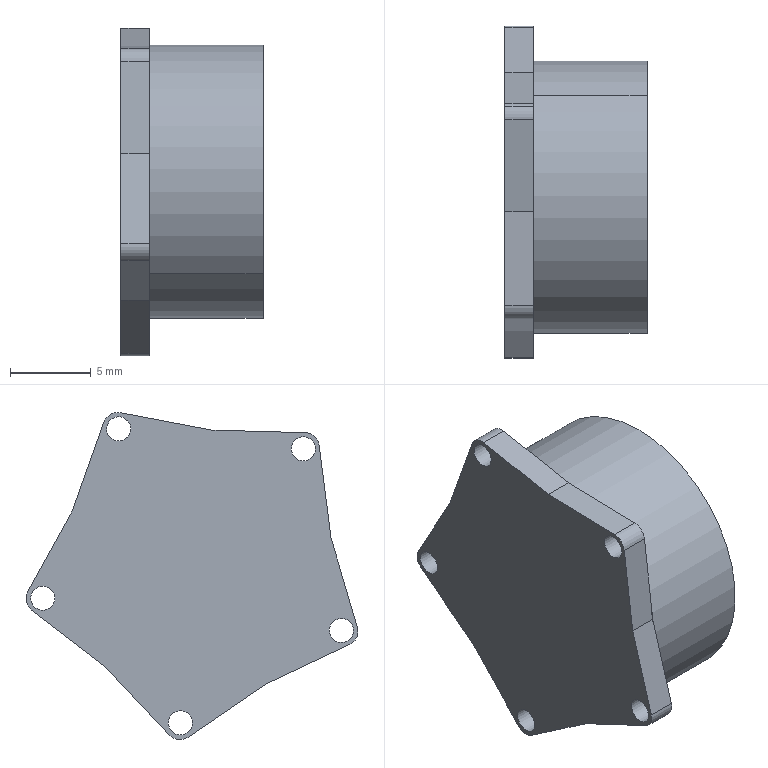Part | SolidWorks | features SplitBody 1 | 1 solid | 101 faces | box 8.8 x 20.538 x 20.245 mm | volume 1206 mm3 | cylinder 55 | cone 24 | plane 22 | commonest cylinder face diameters 0.739 x24 1.496 x10 1.76 x6 2.464 x3 3.52 x2 7.392 x2